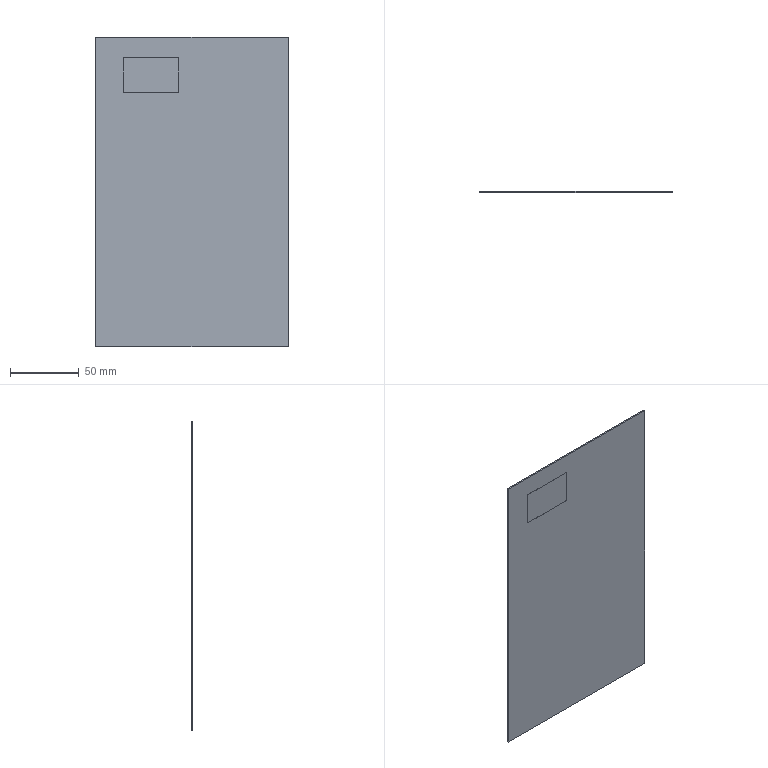Part | STEP file | Computer chassis front-side small door RR | 1 solid | 11 faces | box 140 x 1 x 225 mm | volume 31400 mm3 | plane 11
STEP:
#1=CARTESIAN_POINT('',(0.,0.,0.));
#2=DIRECTION('',(0.,0.,1.));
#3=DIRECTION('',(1.,0.,0.));
#4=AXIS2_PLACEMENT_3D('',#1,#2,#3);
#5=CARTESIAN_POINT('',(70.,1.,-112.5));
#6=VERTEX_POINT('',#5);
#7=CARTESIAN_POINT('',(-70.,1.,-112.5));
#8=VERTEX_POINT('',#7);
#9=CARTESIAN_POINT('',(0.,1.,-112.5));
#10=DIRECTION('',(-1.,0.,0.));
#11=VECTOR('',#10,1.);
#12=LINE('',#9,#11);
#13=CARTESIAN_POINT('',(0.,1.,0.));
#14=DIRECTION('',(0.,1.,0.));
#15=DIRECTION('',(0.,0.,1.));
#16=AXIS2_PLACEMENT_3D('',#13,#14,#15);
#17=PLANE('',#16);
#18=CARTESIAN_POINT('',(-112.5,0.));
#19=DIRECTION('',(0.,-1.));
#20=VECTOR('',#19,1.);
#21=LINE('',#18,#20);
#22=(GEOMETRIC_REPRESENTATION_CONTEXT(2)PARAMETRIC_REPRESENTATION_CONTEXT()REPRESENTATION_CONTEXT('',''));
#23=DEFINITIONAL_REPRESENTATION('',(#21),#22);
#24=PCURVE('',#17,#23);
#25=CARTESIAN_POINT('',(70.,0.,-112.5));
#26=DIRECTION('',(0.,0.,-1.));
#27=DIRECTION('',(-1.,0.,0.));
#28=AXIS2_PLACEMENT_3D('',#25,#26,#27);
#29=PLANE('',#28);
#30=CARTESIAN_POINT('',(70.,1.));
#31=DIRECTION('',(1.,0.));
#32=VECTOR('',#31,1.);
#33=LINE('',#30,#32);
#34=(GEOMETRIC_REPRESENTATION_CONTEXT(2)PARAMETRIC_REPRESENTATION_CONTEXT()REPRESENTATION_CONTEXT('',''));
#35=DEFINITIONAL_REPRESENTATION('',(#33),#34);
#36=PCURVE('',#29,#35);
#37=SURFACE_CURVE('',#12,(#24,#36),.PCURVE_S1.);
#38=EDGE_CURVE('',#6,#8,#37,.T.);
#39=ORIENTED_EDGE('',*,*,#38,.T.);
#40=CARTESIAN_POINT('',(-70.,1.,112.5));
#41=VERTEX_POINT('',#40);
#42=CARTESIAN_POINT('',(-70.,1.,0.));
#43=DIRECTION('',(0.,0.,1.));
#44=VECTOR('',#43,1.);
#45=LINE('',#42,#44);
#46=CARTESIAN_POINT('',(0.,-70.));
#47=DIRECTION('',(1.,0.));
#48=VECTOR('',#47,1.);
#49=LINE('',#46,#48);
#50=(GEOMETRIC_REPRESENTATION_CONTEXT(2)PARAMETRIC_REPRESENTATION_CONTEXT()REPRESENTATION_CONTEXT('',''));
#51=DEFINITIONAL_REPRESENTATION('',(#49),#50);
#52=PCURVE('',#17,#51);
#53=CARTESIAN_POINT('',(-70.,0.,-112.5));
#54=DIRECTION('',(-1.,0.,0.));
#55=DIRECTION('',(0.,0.,1.));
#56=AXIS2_PLACEMENT_3D('',#53,#54,#55);
#57=PLANE('',#56);
#58=CARTESIAN_POINT('',(112.5,1.));
#59=DIRECTION('',(1.,0.));
#60=VECTOR('',#59,1.);
#61=LINE('',#58,#60);
#62=(GEOMETRIC_REPRESENTATION_CONTEXT(2)PARAMETRIC_REPRESENTATION_CONTEXT()REPRESENTATION_CONTEXT('',''));
#63=DEFINITIONAL_REPRESENTATION('',(#61),#62);
#64=PCURVE('',#57,#63);
#65=SURFACE_CURVE('',#45,(#52,#64),.PCURVE_S1.);
#66=EDGE_CURVE('',#8,#41,#65,.T.);
#67=ORIENTED_EDGE('',*,*,#66,.T.);
#68=CARTESIAN_POINT('',(70.,1.,112.5));
#69=VERTEX_POINT('',#68);
#70=CARTESIAN_POINT('',(0.,1.,112.5));
#71=DIRECTION('',(1.,0.,0.));
#72=VECTOR('',#71,1.);
#73=LINE('',#70,#72);
#74=CARTESIAN_POINT('',(112.5,0.));
#75=DIRECTION('',(0.,1.));
#76=VECTOR('',#75,1.);
#77=LINE('',#74,#76);
#78=(GEOMETRIC_REPRESENTATION_CONTEXT(2)PARAMETRIC_REPRESENTATION_CONTEXT()REPRESENTATION_CONTEXT('',''));
#79=DEFINITIONAL_REPRESENTATION('',(#77),#78);
#80=PCURVE('',#17,#79);
#81=CARTESIAN_POINT('',(-70.,0.,112.5));
#82=DIRECTION('',(0.,0.,1.));
#83=DIRECTION('',(1.,0.,0.));
#84=AXIS2_PLACEMENT_3D('',#81,#82,#83);
#85=PLANE('',#84);
#86=CARTESIAN_POINT('',(70.,1.));
#87=DIRECTION('',(1.,0.));
#88=VECTOR('',#87,1.);
#89=LINE('',#86,#88);
#90=(GEOMETRIC_REPRESENTATION_CONTEXT(2)PARAMETRIC_REPRESENTATION_CONTEXT()REPRESENTATION_CONTEXT('',''));
#91=DEFINITIONAL_REPRESENTATION('',(#89),#90);
#92=PCURVE('',#85,#91);
#93=SURFACE_CURVE('',#73,(#80,#92),.PCURVE_S1.);
#94=EDGE_CURVE('',#41,#69,#93,.T.);
#95=ORIENTED_EDGE('',*,*,#94,.T.);
#96=CARTESIAN_POINT('',(70.,1.,0.));
#97=DIRECTION('',(0.,0.,-1.));
#98=VECTOR('',#97,1.);
#99=LINE('',#96,#98);
#100=CARTESIAN_POINT('',(0.,70.));
#101=DIRECTION('',(-1.,0.));
#102=VECTOR('',#101,1.);
#103=LINE('',#100,#102);
#104=(GEOMETRIC_REPRESENTATION_CONTEXT(2)PARAMETRIC_REPRESENTATION_CONTEXT()REPRESENTATION_CONTEXT('',''));
#105=DEFINITIONAL_REPRESENTATION('',(#103),#104);
#106=PCURVE('',#17,#105);
#107=CARTESIAN_POINT('',(70.,0.,112.5));
#108=DIRECTION('',(1.,0.,0.));
#109=DIRECTION('',(0.,0.,-1.));
#110=AXIS2_PLACEMENT_3D('',#107,#108,#109);
#111=PLANE('',#110);
#112=CARTESIAN_POINT('',(112.5,1.));
#113=DIRECTION('',(1.,0.));
#114=VECTOR('',#113,1.);
#115=LINE('',#112,#114);
#116=(GEOMETRIC_REPRESENTATION_CONTEXT(2)PARAMETRIC_REPRESENTATION_CONTEXT()REPRESENTATION_CONTEXT('',''));
#117=DEFINITIONAL_REPRESENTATION('',(#115),#116);
#118=PCURVE('',#111,#117);
#119=SURFACE_CURVE('',#99,(#106,#118),.PCURVE_S1.);
#120=EDGE_CURVE('',#69,#6,#119,.T.);
#121=ORIENTED_EDGE('',*,*,#120,.T.);
#122=EDGE_LOOP('',(#39,#67,#95,#121));
#123=FACE_BOUND('',#122,.T.);
#124=ADVANCED_FACE('',(#123),#17,.T.);
#125=CARTESIAN_POINT('',(-70.,0.,-112.5));
#126=VERTEX_POINT('',#125);
#127=CARTESIAN_POINT('',(-70.,0.,-112.5));
#128=DIRECTION('',(0.,-1.,0.));
#129=VECTOR('',#128,1.);
#130=LINE('',#127,#129);
#131=CARTESIAN_POINT('',(0.,0.));
#132=DIRECTION('',(0.,-1.));
#133=VECTOR('',#132,1.);
#134=LINE('',#131,#133);
#135=(GEOMETRIC_REPRESENTATION_CONTEXT(2)PARAMETRIC_REPRESENTATION_CONTEXT()REPRESENTATION_CONTEXT('',''));
#136=DEFINITIONAL_REPRESENTATION('',(#134),#135);
#137=PCURVE('',#57,#136);
#138=CARTESIAN_POINT('',(140.,0.));
#139=DIRECTION('',(0.,-1.));
#140=VECTOR('',#139,1.);
#141=LINE('',#138,#140);
#142=(GEOMETRIC_REPRESENTATION_CONTEXT(2)PARAMETRIC_REPRESENTATION_CONTEXT()REPRESENTATION_CONTEXT('',''));
#143=DEFINITIONAL_REPRESENTATION('',(#141),#142);
#144=PCURVE('',#29,#143);
#145=SURFACE_CURVE('',#130,(#137,#144),.PCURVE_S1.);
#146=EDGE_CURVE('',#8,#126,#145,.T.);
#147=ORIENTED_EDGE('',*,*,#146,.T.);
#148=CARTESIAN_POINT('',(-70.,0.,112.5));
#149=VERTEX_POINT('',#148);
#150=CARTESIAN_POINT('',(-70.,0.,-112.5));
#151=DIRECTION('',(0.,0.,1.));
#152=VECTOR('',#151,1.);
#153=LINE('',#150,#152);
#154=CARTESIAN_POINT('',(0.,0.));
#155=DIRECTION('',(1.,0.));
#156=VECTOR('',#155,1.);
#157=LINE('',#154,#156);
#158=(GEOMETRIC_REPRESENTATION_CONTEXT(2)PARAMETRIC_REPRESENTATION_CONTEXT()REPRESENTATION_CONTEXT('',''));
#159=DEFINITIONAL_REPRESENTATION('',(#157),#158);
#160=PCURVE('',#57,#159);
#161=CARTESIAN_POINT('',(0.,0.,0.));
#162=DIRECTION('',(0.,1.,0.));
#163=DIRECTION('',(0.,0.,1.));
#164=AXIS2_PLACEMENT_3D('',#161,#162,#163);
#165=PLANE('',#164);
#166=CARTESIAN_POINT('',(-112.5,-70.));
#167=DIRECTION('',(1.,0.));
#168=VECTOR('',#167,1.);
#169=LINE('',#166,#168);
#170=(GEOMETRIC_REPRESENTATION_CONTEXT(2)PARAMETRIC_REPRESENTATION_CONTEXT()REPRESENTATION_CONTEXT('',''));
#171=DEFINITIONAL_REPRESENTATION('',(#169),#170);
#172=PCURVE('',#165,#171);
#173=SURFACE_CURVE('',#153,(#160,#172),.PCURVE_S1.);
#174=EDGE_CURVE('',#126,#149,#173,.T.);
#175=ORIENTED_EDGE('',*,*,#174,.T.);
#176=CARTESIAN_POINT('',(-70.,0.,112.5));
#177=DIRECTION('',(0.,1.,0.));
#178=VECTOR('',#177,1.);
#179=LINE('',#176,#178);
#180=CARTESIAN_POINT('',(225.,0.));
#181=DIRECTION('',(0.,1.));
#182=VECTOR('',#181,1.);
#183=LINE('',#180,#182);
#184=(GEOMETRIC_REPRESENTATION_CONTEXT(2)PARAMETRIC_REPRESENTATION_CONTEXT()REPRESENTATION_CONTEXT('',''));
#185=DEFINITIONAL_REPRESENTATION('',(#183),#184);
#186=PCURVE('',#57,#185);
#187=CARTESIAN_POINT('',(0.,0.));
#188=DIRECTION('',(0.,1.));
#189=VECTOR('',#188,1.);
#190=LINE('',#187,#189);
#191=(GEOMETRIC_REPRESENTATION_CONTEXT(2)PARAMETRIC_REPRESENTATION_CONTEXT()REPRESENTATION_CONTEXT('',''));
#192=DEFINITIONAL_REPRESENTATION('',(#190),#191);
#193=PCURVE('',#85,#192);
#194=SURFACE_CURVE('',#179,(#186,#193),.PCURVE_S1.);
#195=EDGE_CURVE('',#149,#41,#194,.T.);
#196=ORIENTED_EDGE('',*,*,#195,.T.);
#197=ORIENTED_EDGE('',*,*,#66,.F.);
#198=EDGE_LOOP('',(#147,#175,#196,#197));
#199=FACE_BOUND('',#198,.T.);
#200=ADVANCED_FACE('',(#199),#57,.T.);
#201=CARTESIAN_POINT('',(70.,0.,-112.5));
#202=VERTEX_POINT('',#201);
#203=CARTESIAN_POINT('',(70.,0.,-112.5));
#204=DIRECTION('',(0.,-1.,0.));
#205=VECTOR('',#204,1.);
#206=LINE('',#203,#205);
#207=CARTESIAN_POINT('',(0.,0.));
#208=DIRECTION('',(0.,-1.));
#209=VECTOR('',#208,1.);
#210=LINE('',#207,#209);
#211=(GEOMETRIC_REPRESENTATION_CONTEXT(2)PARAMETRIC_REPRESENTATION_CONTEXT()REPRESENTATION_CONTEXT('',''));
#212=DEFINITIONAL_REPRESENTATION('',(#210),#211);
#213=PCURVE('',#29,#212);
#214=CARTESIAN_POINT('',(225.,0.));
#215=DIRECTION('',(0.,-1.));
#216=VECTOR('',#215,1.);
#217=LINE('',#214,#216);
#218=(GEOMETRIC_REPRESENTATION_CONTEXT(2)PARAMETRIC_REPRESENTATION_CONTEXT()REPRESENTATION_CONTEXT('',''));
#219=DEFINITIONAL_REPRESENTATION('',(#217),#218);
#220=PCURVE('',#111,#219);
#221=SURFACE_CURVE('',#206,(#213,#220),.PCURVE_S1.);
#222=EDGE_CURVE('',#6,#202,#221,.T.);
#223=ORIENTED_EDGE('',*,*,#222,.T.);
#224=CARTESIAN_POINT('',(70.,0.,-112.5));
#225=DIRECTION('',(-1.,0.,0.));
#226=VECTOR('',#225,1.);
#227=LINE('',#224,#226);
#228=CARTESIAN_POINT('',(0.,0.));
#229=DIRECTION('',(1.,0.));
#230=VECTOR('',#229,1.);
#231=LINE('',#228,#230);
#232=(GEOMETRIC_REPRESENTATION_CONTEXT(2)PARAMETRIC_REPRESENTATION_CONTEXT()REPRESENTATION_CONTEXT('',''));
#233=DEFINITIONAL_REPRESENTATION('',(#231),#232);
#234=PCURVE('',#29,#233);
#235=CARTESIAN_POINT('',(-112.5,70.));
#236=DIRECTION('',(0.,-1.));
#237=VECTOR('',#236,1.);
#238=LINE('',#235,#237);
#239=(GEOMETRIC_REPRESENTATION_CONTEXT(2)PARAMETRIC_REPRESENTATION_CONTEXT()REPRESENTATION_CONTEXT('',''));
#240=DEFINITIONAL_REPRESENTATION('',(#238),#239);
#241=PCURVE('',#165,#240);
#242=SURFACE_CURVE('',#227,(#234,#241),.PCURVE_S1.);
#243=EDGE_CURVE('',#202,#126,#242,.T.);
#244=ORIENTED_EDGE('',*,*,#243,.T.);
#245=ORIENTED_EDGE('',*,*,#146,.F.);
#246=ORIENTED_EDGE('',*,*,#38,.F.);
#247=EDGE_LOOP('',(#223,#244,#245,#246));
#248=FACE_BOUND('',#247,.T.);
#249=ADVANCED_FACE('',(#248),#29,.T.);
#250=CARTESIAN_POINT('',(70.,0.,112.5));
#251=VERTEX_POINT('',#250);
#252=CARTESIAN_POINT('',(70.,0.,112.5));
#253=DIRECTION('',(0.,-1.,0.));
#254=VECTOR('',#253,1.);
#255=LINE('',#252,#254);
#256=CARTESIAN_POINT('',(0.,0.));
#257=DIRECTION('',(0.,-1.));
#258=VECTOR('',#257,1.);
#259=LINE('',#256,#258);
#260=(GEOMETRIC_REPRESENTATION_CONTEXT(2)PARAMETRIC_REPRESENTATION_CONTEXT()REPRESENTATION_CONTEXT('',''));
#261=DEFINITIONAL_REPRESENTATION('',(#259),#260);
#262=PCURVE('',#111,#261);
#263=CARTESIAN_POINT('',(140.,0.));
#264=DIRECTION('',(0.,-1.));
#265=VECTOR('',#264,1.);
#266=LINE('',#263,#265);
#267=(GEOMETRIC_REPRESENTATION_CONTEXT(2)PARAMETRIC_REPRESENTATION_CONTEXT()REPRESENTATION_CONTEXT('',''));
#268=DEFINITIONAL_REPRESENTATION('',(#266),#267);
#269=PCURVE('',#85,#268);
#270=SURFACE_CURVE('',#255,(#262,#269),.PCURVE_S1.);
#271=EDGE_CURVE('',#69,#251,#270,.T.);
#272=ORIENTED_EDGE('',*,*,#271,.T.);
#273=CARTESIAN_POINT('',(70.,0.,112.5));
#274=DIRECTION('',(0.,0.,-1.));
#275=VECTOR('',#274,1.);
#276=LINE('',#273,#275);
#277=CARTESIAN_POINT('',(0.,0.));
#278=DIRECTION('',(1.,0.));
#279=VECTOR('',#278,1.);
#280=LINE('',#277,#279);
#281=(GEOMETRIC_REPRESENTATION_CONTEXT(2)PARAMETRIC_REPRESENTATION_CONTEXT()REPRESENTATION_CONTEXT('',''));
#282=DEFINITIONAL_REPRESENTATION('',(#280),#281);
#283=PCURVE('',#111,#282);
#284=CARTESIAN_POINT('',(112.5,70.));
#285=DIRECTION('',(-1.,0.));
#286=VECTOR('',#285,1.);
#287=LINE('',#284,#286);
#288=(GEOMETRIC_REPRESENTATION_CONTEXT(2)PARAMETRIC_REPRESENTATION_CONTEXT()REPRESENTATION_CONTEXT('',''));
#289=DEFINITIONAL_REPRESENTATION('',(#287),#288);
#290=PCURVE('',#165,#289);
#291=SURFACE_CURVE('',#276,(#283,#290),.PCURVE_S1.);
#292=EDGE_CURVE('',#251,#202,#291,.T.);
#293=ORIENTED_EDGE('',*,*,#292,.T.);
#294=ORIENTED_EDGE('',*,*,#222,.F.);
#295=ORIENTED_EDGE('',*,*,#120,.F.);
#296=EDGE_LOOP('',(#272,#293,#294,#295));
#297=FACE_BOUND('',#296,.T.);
#298=ADVANCED_FACE('',(#297),#111,.T.);
#299=ORIENTED_EDGE('',*,*,#195,.F.);
#300=CARTESIAN_POINT('',(-70.,0.,112.5));
#301=DIRECTION('',(1.,0.,0.));
#302=VECTOR('',#301,1.);
#303=LINE('',#300,#302);
#304=CARTESIAN_POINT('',(0.,0.));
#305=DIRECTION('',(1.,0.));
#306=VECTOR('',#305,1.);
#307=LINE('',#304,#306);
#308=(GEOMETRIC_REPRESENTATION_CONTEXT(2)PARAMETRIC_REPRESENTATION_CONTEXT()REPRESENTATION_CONTEXT('',''));
#309=DEFINITIONAL_REPRESENTATION('',(#307),#308);
#310=PCURVE('',#85,#309);
#311=CARTESIAN_POINT('',(112.5,-70.));
#312=DIRECTION('',(0.,1.));
#313=VECTOR('',#312,1.);
#314=LINE('',#311,#313);
#315=(GEOMETRIC_REPRESENTATION_CONTEXT(2)PARAMETRIC_REPRESENTATION_CONTEXT()REPRESENTATION_CONTEXT('',''));
#316=DEFINITIONAL_REPRESENTATION('',(#314),#315);
#317=PCURVE('',#165,#316);
#318=SURFACE_CURVE('',#303,(#310,#317),.PCURVE_S1.);
#319=EDGE_CURVE('',#149,#251,#318,.T.);
#320=ORIENTED_EDGE('',*,*,#319,.T.);
#321=ORIENTED_EDGE('',*,*,#271,.F.);
#322=ORIENTED_EDGE('',*,*,#94,.F.);
#323=EDGE_LOOP('',(#299,#320,#321,#322));
#324=FACE_BOUND('',#323,.T.);
#325=ADVANCED_FACE('',(#324),#85,.T.);
#326=CARTESIAN_POINT('',(-50.,0.,97.5));
#327=VERTEX_POINT('',#326);
#328=CARTESIAN_POINT('',(-50.,0.,72.5));
#329=VERTEX_POINT('',#328);
#330=CARTESIAN_POINT('',(-50.,0.,0.));
#331=DIRECTION('',(0.,0.,-1.));
#332=VECTOR('',#331,1.);
#333=LINE('',#330,#332);
#334=CARTESIAN_POINT('',(0.,-50.));
#335=DIRECTION('',(-1.,0.));
#336=VECTOR('',#335,1.);
#337=LINE('',#334,#336);
#338=(GEOMETRIC_REPRESENTATION_CONTEXT(2)PARAMETRIC_REPRESENTATION_CONTEXT()REPRESENTATION_CONTEXT('',''));
#339=DEFINITIONAL_REPRESENTATION('',(#337),#338);
#340=PCURVE('',#165,#339);
#341=CARTESIAN_POINT('',(-50.,0.,97.5));
#342=DIRECTION('',(-1.,0.,0.));
#343=DIRECTION('',(0.,0.,1.));
#344=AXIS2_PLACEMENT_3D('',#341,#342,#343);
#345=PLANE('',#344);
#346=CARTESIAN_POINT('',(-97.5,0.));
#347=DIRECTION('',(-1.,0.));
#348=VECTOR('',#347,1.);
#349=LINE('',#346,#348);
#350=(GEOMETRIC_REPRESENTATION_CONTEXT(2)PARAMETRIC_REPRESENTATION_CONTEXT()REPRESENTATION_CONTEXT('',''));
#351=DEFINITIONAL_REPRESENTATION('',(#349),#350);
#352=PCURVE('',#345,#351);
#353=SURFACE_CURVE('',#333,(#340,#352),.PCURVE_S1.);
#354=EDGE_CURVE('',#327,#329,#353,.T.);
#355=ORIENTED_EDGE('',*,*,#354,.F.);
#356=CARTESIAN_POINT('',(-10.,0.,97.5));
#357=VERTEX_POINT('',#356);
#358=CARTESIAN_POINT('',(0.,0.,97.5));
#359=DIRECTION('',(-1.,0.,0.));
#360=VECTOR('',#359,1.);
#361=LINE('',#358,#360);
#362=CARTESIAN_POINT('',(97.5,0.));
#363=DIRECTION('',(0.,-1.));
#364=VECTOR('',#363,1.);
#365=LINE('',#362,#364);
#366=(GEOMETRIC_REPRESENTATION_CONTEXT(2)PARAMETRIC_REPRESENTATION_CONTEXT()REPRESENTATION_CONTEXT('',''));
#367=DEFINITIONAL_REPRESENTATION('',(#365),#366);
#368=PCURVE('',#165,#367);
#369=CARTESIAN_POINT('',(-10.,0.,97.5));
#370=DIRECTION('',(0.,0.,1.));
#371=DIRECTION('',(1.,0.,0.));
#372=AXIS2_PLACEMENT_3D('',#369,#370,#371);
#373=PLANE('',#372);
#374=CARTESIAN_POINT('',(10.,0.));
#375=DIRECTION('',(-1.,0.));
#376=VECTOR('',#375,1.);
#377=LINE('',#374,#376);
#378=(GEOMETRIC_REPRESENTATION_CONTEXT(2)PARAMETRIC_REPRESENTATION_CONTEXT()REPRESENTATION_CONTEXT('',''));
#379=DEFINITIONAL_REPRESENTATION('',(#377),#378);
#380=PCURVE('',#373,#379);
#381=SURFACE_CURVE('',#361,(#368,#380),.PCURVE_S1.);
#382=EDGE_CURVE('',#357,#327,#381,.T.);
#383=ORIENTED_EDGE('',*,*,#382,.F.);
#384=CARTESIAN_POINT('',(-10.,0.,72.5));
#385=VERTEX_POINT('',#384);
#386=CARTESIAN_POINT('',(-10.,0.,0.));
#387=DIRECTION('',(0.,0.,1.));
#388=VECTOR('',#387,1.);
#389=LINE('',#386,#388);
#390=CARTESIAN_POINT('',(0.,-10.));
#391=DIRECTION('',(1.,0.));
#392=VECTOR('',#391,1.);
#393=LINE('',#390,#392);
#394=(GEOMETRIC_REPRESENTATION_CONTEXT(2)PARAMETRIC_REPRESENTATION_CONTEXT()REPRESENTATION_CONTEXT('',''));
#395=DEFINITIONAL_REPRESENTATION('',(#393),#394);
#396=PCURVE('',#165,#395);
#397=CARTESIAN_POINT('',(-10.,0.,72.5));
#398=DIRECTION('',(1.,0.,0.));
#399=DIRECTION('',(0.,0.,-1.));
#400=AXIS2_PLACEMENT_3D('',#397,#398,#399);
#401=PLANE('',#400);
#402=CARTESIAN_POINT('',(72.5,0.));
#403=DIRECTION('',(-1.,0.));
#404=VECTOR('',#403,1.);
#405=LINE('',#402,#404);
#406=(GEOMETRIC_REPRESENTATION_CONTEXT(2)PARAMETRIC_REPRESENTATION_CONTEXT()REPRESENTATION_CONTEXT('',''));
#407=DEFINITIONAL_REPRESENTATION('',(#405),#406);
#408=PCURVE('',#401,#407);
#409=SURFACE_CURVE('',#389,(#396,#408),.PCURVE_S1.);
#410=EDGE_CURVE('',#385,#357,#409,.T.);
#411=ORIENTED_EDGE('',*,*,#410,.F.);
#412=CARTESIAN_POINT('',(0.,0.,72.5));
#413=DIRECTION('',(1.,0.,0.));
#414=VECTOR('',#413,1.);
#415=LINE('',#412,#414);
#416=CARTESIAN_POINT('',(72.5,0.));
#417=DIRECTION('',(0.,1.));
#418=VECTOR('',#417,1.);
#419=LINE('',#416,#418);
#420=(GEOMETRIC_REPRESENTATION_CONTEXT(2)PARAMETRIC_REPRESENTATION_CONTEXT()REPRESENTATION_CONTEXT('',''));
#421=DEFINITIONAL_REPRESENTATION('',(#419),#420);
#422=PCURVE('',#165,#421);
#423=CARTESIAN_POINT('',(-50.,0.,72.5));
#424=DIRECTION('',(0.,0.,-1.));
#425=DIRECTION('',(-1.,0.,0.));
#426=AXIS2_PLACEMENT_3D('',#423,#424,#425);
#427=PLANE('',#426);
#428=CARTESIAN_POINT('',(-50.,0.));
#429=DIRECTION('',(-1.,0.));
#430=VECTOR('',#429,1.);
#431=LINE('',#428,#430);
#432=(GEOMETRIC_REPRESENTATION_CONTEXT(2)PARAMETRIC_REPRESENTATION_CONTEXT()REPRESENTATION_CONTEXT('',''));
#433=DEFINITIONAL_REPRESENTATION('',(#431),#432);
#434=PCURVE('',#427,#433);
#435=SURFACE_CURVE('',#415,(#422,#434),.PCURVE_S1.);
#436=EDGE_CURVE('',#329,#385,#435,.T.);
#437=ORIENTED_EDGE('',*,*,#436,.F.);
#438=EDGE_LOOP('',(#355,#383,#411,#437));
#439=FACE_BOUND('',#438,.T.);
#440=ORIENTED_EDGE('',*,*,#292,.F.);
#441=ORIENTED_EDGE('',*,*,#319,.F.);
#442=ORIENTED_EDGE('',*,*,#174,.F.);
#443=ORIENTED_EDGE('',*,*,#243,.F.);
#444=EDGE_LOOP('',(#440,#441,#442,#443));
#445=FACE_BOUND('',#444,.T.);
#446=ADVANCED_FACE('',(#439,#445),#165,.F.);
#447=CARTESIAN_POINT('',(-50.,0.1,72.5));
#448=VERTEX_POINT('',#447);
#449=CARTESIAN_POINT('',(-10.,0.1,72.5));
#450=VERTEX_POINT('',#449);
#451=CARTESIAN_POINT('',(-50.,0.1,72.5));
#452=DIRECTION('',(1.,0.,0.));
#453=VECTOR('',#452,1.);
#454=LINE('',#451,#453);
#455=CARTESIAN_POINT('',(0.,0.1));
#456=DIRECTION('',(-1.,0.));
#457=VECTOR('',#456,1.);
#458=LINE('',#455,#457);
#459=(GEOMETRIC_REPRESENTATION_CONTEXT(2)PARAMETRIC_REPRESENTATION_CONTEXT()REPRESENTATION_CONTEXT('',''));
#460=DEFINITIONAL_REPRESENTATION('',(#458),#459);
#461=PCURVE('',#427,#460);
#462=CARTESIAN_POINT('',(0.,0.1,0.));
#463=DIRECTION('',(0.,-1.,0.));
#464=DIRECTION('',(0.,0.,-1.));
#465=AXIS2_PLACEMENT_3D('',#462,#463,#464);
#466=PLANE('',#465);
#467=CARTESIAN_POINT('',(-72.5,-50.));
#468=DIRECTION('',(0.,1.));
#469=VECTOR('',#468,1.);
#470=LINE('',#467,#469);
#471=(GEOMETRIC_REPRESENTATION_CONTEXT(2)PARAMETRIC_REPRESENTATION_CONTEXT()REPRESENTATION_CONTEXT('',''));
#472=DEFINITIONAL_REPRESENTATION('',(#470),#471);
#473=PCURVE('',#466,#472);
#474=SURFACE_CURVE('',#454,(#461,#473),.PCURVE_S1.);
#475=EDGE_CURVE('',#448,#450,#474,.T.);
#476=ORIENTED_EDGE('',*,*,#475,.F.);
#477=CARTESIAN_POINT('',(-50.,0.,72.5));
#478=DIRECTION('',(0.,1.,0.));
#479=VECTOR('',#478,1.);
#480=LINE('',#477,#479);
#481=CARTESIAN_POINT('',(0.,0.));
#482=DIRECTION('',(0.,1.));
#483=VECTOR('',#482,1.);
#484=LINE('',#481,#483);
#485=(GEOMETRIC_REPRESENTATION_CONTEXT(2)PARAMETRIC_REPRESENTATION_CONTEXT()REPRESENTATION_CONTEXT('',''));
#486=DEFINITIONAL_REPRESENTATION('',(#484),#485);
#487=PCURVE('',#427,#486);
#488=CARTESIAN_POINT('',(-25.,0.));
#489=DIRECTION('',(0.,1.));
#490=VECTOR('',#489,1.);
#491=LINE('',#488,#490);
#492=(GEOMETRIC_REPRESENTATION_CONTEXT(2)PARAMETRIC_REPRESENTATION_CONTEXT()REPRESENTATION_CONTEXT('',''));
#493=DEFINITIONAL_REPRESENTATION('',(#491),#492);
#494=PCURVE('',#345,#493);
#495=SURFACE_CURVE('',#480,(#487,#494),.PCURVE_S1.);
#496=EDGE_CURVE('',#329,#448,#495,.T.);
#497=ORIENTED_EDGE('',*,*,#496,.F.);
#498=ORIENTED_EDGE('',*,*,#436,.T.);
#499=CARTESIAN_POINT('',(-10.,0.,72.5));
#500=DIRECTION('',(0.,-1.,0.));
#501=VECTOR('',#500,1.);
#502=LINE('',#499,#501);
#503=CARTESIAN_POINT('',(-40.,0.));
#504=DIRECTION('',(0.,-1.));
#505=VECTOR('',#504,1.);
#506=LINE('',#503,#505);
#507=(GEOMETRIC_REPRESENTATION_CONTEXT(2)PARAMETRIC_REPRESENTATION_CONTEXT()REPRESENTATION_CONTEXT('',''));
#508=DEFINITIONAL_REPRESENTATION('',(#506),#507);
#509=PCURVE('',#427,#508);
#510=CARTESIAN_POINT('',(0.,0.));
#511=DIRECTION('',(0.,-1.));
#512=VECTOR('',#511,1.);
#513=LINE('',#510,#512);
#514=(GEOMETRIC_REPRESENTATION_CONTEXT(2)PARAMETRIC_REPRESENTATION_CONTEXT()REPRESENTATION_CONTEXT('',''));
#515=DEFINITIONAL_REPRESENTATION('',(#513),#514);
#516=PCURVE('',#401,#515);
#517=SURFACE_CURVE('',#502,(#509,#516),.PCURVE_S1.);
#518=EDGE_CURVE('',#450,#385,#517,.T.);
#519=ORIENTED_EDGE('',*,*,#518,.F.);
#520=EDGE_LOOP('',(#476,#497,#498,#519));
#521=FACE_BOUND('',#520,.T.);
#522=ADVANCED_FACE('',(#521),#427,.F.);
#523=CARTESIAN_POINT('',(-50.,0.1,97.5));
#524=VERTEX_POINT('',#523);
#525=CARTESIAN_POINT('',(-50.,0.1,97.5));
#526=DIRECTION('',(0.,0.,-1.));
#527=VECTOR('',#526,1.);
#528=LINE('',#525,#527);
#529=CARTESIAN_POINT('',(0.,0.1));
#530=DIRECTION('',(-1.,0.));
#531=VECTOR('',#530,1.);
#532=LINE('',#529,#531);
#533=(GEOMETRIC_REPRESENTATION_CONTEXT(2)PARAMETRIC_REPRESENTATION_CONTEXT()REPRESENTATION_CONTEXT('',''));
#534=DEFINITIONAL_REPRESENTATION('',(#532),#533);
#535=PCURVE('',#345,#534);
#536=CARTESIAN_POINT('',(-97.5,-50.));
#537=DIRECTION('',(1.,0.));
#538=VECTOR('',#537,1.);
#539=LINE('',#536,#538);
#540=(GEOMETRIC_REPRESENTATION_CONTEXT(2)PARAMETRIC_REPRESENTATION_CONTEXT()REPRESENTATION_CONTEXT('',''));
#541=DEFINITIONAL_REPRESENTATION('',(#539),#540);
#542=PCURVE('',#466,#541);
#543=SURFACE_CURVE('',#528,(#535,#542),.PCURVE_S1.);
#544=EDGE_CURVE('',#524,#448,#543,.T.);
#545=ORIENTED_EDGE('',*,*,#544,.F.);
#546=CARTESIAN_POINT('',(-50.,0.,97.5));
#547=DIRECTION('',(0.,1.,0.));
#548=VECTOR('',#547,1.);
#549=LINE('',#546,#548);
#550=CARTESIAN_POINT('',(0.,0.));
#551=DIRECTION('',(0.,1.));
#552=VECTOR('',#551,1.);
#553=LINE('',#550,#552);
#554=(GEOMETRIC_REPRESENTATION_CONTEXT(2)PARAMETRIC_REPRESENTATION_CONTEXT()REPRESENTATION_CONTEXT('',''));
#555=DEFINITIONAL_REPRESENTATION('',(#553),#554);
#556=PCURVE('',#345,#555);
#557=CARTESIAN_POINT('',(-40.,0.));
#558=DIRECTION('',(0.,1.));
#559=VECTOR('',#558,1.);
#560=LINE('',#557,#559);
#561=(GEOMETRIC_REPRESENTATION_CONTEXT(2)PARAMETRIC_REPRESENTATION_CONTEXT()REPRESENTATION_CONTEXT('',''));
#562=DEFINITIONAL_REPRESENTATION('',(#560),#561);
#563=PCURVE('',#373,#562);
#564=SURFACE_CURVE('',#549,(#556,#563),.PCURVE_S1.);
#565=EDGE_CURVE('',#327,#524,#564,.T.);
#566=ORIENTED_EDGE('',*,*,#565,.F.);
#567=ORIENTED_EDGE('',*,*,#354,.T.);
#568=ORIENTED_EDGE('',*,*,#496,.T.);
#569=EDGE_LOOP('',(#545,#566,#567,#568));
#570=FACE_BOUND('',#569,.T.);
#571=ADVANCED_FACE('',(#570),#345,.F.);
#572=CARTESIAN_POINT('',(-10.,0.1,97.5));
#573=VERTEX_POINT('',#572);
#574=CARTESIAN_POINT('',(-10.,0.1,97.5));
#575=DIRECTION('',(-1.,0.,0.));
#576=VECTOR('',#575,1.);
#577=LINE('',#574,#576);
#578=CARTESIAN_POINT('',(0.,0.1));
#579=DIRECTION('',(-1.,0.));
#580=VECTOR('',#579,1.);
#581=LINE('',#578,#580);
#582=(GEOMETRIC_REPRESENTATION_CONTEXT(2)PARAMETRIC_REPRESENTATION_CONTEXT()REPRESENTATION_CONTEXT('',''));
#583=DEFINITIONAL_REPRESENTATION('',(#581),#582);
#584=PCURVE('',#373,#583);
#585=CARTESIAN_POINT('',(-97.5,-10.));
#586=DIRECTION('',(0.,-1.));
#587=VECTOR('',#586,1.);
#588=LINE('',#585,#587);
#589=(GEOMETRIC_REPRESENTATION_CONTEXT(2)PARAMETRIC_REPRESENTATION_CONTEXT()REPRESENTATION_CONTEXT('',''));
#590=DEFINITIONAL_REPRESENTATION('',(#588),#589);
#591=PCURVE('',#466,#590);
#592=SURFACE_CURVE('',#577,(#584,#591),.PCURVE_S1.);
#593=EDGE_CURVE('',#573,#524,#592,.T.);
#594=ORIENTED_EDGE('',*,*,#593,.F.);
#595=CARTESIAN_POINT('',(-10.,0.,97.5));
#596=DIRECTION('',(0.,1.,0.));
#597=VECTOR('',#596,1.);
#598=LINE('',#595,#597);
#599=CARTESIAN_POINT('',(0.,0.));
#600=DIRECTION('',(0.,1.));
#601=VECTOR('',#600,1.);
#602=LINE('',#599,#601);
#603=(GEOMETRIC_REPRESENTATION_CONTEXT(2)PARAMETRIC_REPRESENTATION_CONTEXT()REPRESENTATION_CONTEXT('',''));
#604=DEFINITIONAL_REPRESENTATION('',(#602),#603);
#605=PCURVE('',#373,#604);
#606=CARTESIAN_POINT('',(-25.,0.));
#607=DIRECTION('',(0.,1.));
#608=VECTOR('',#607,1.);
#609=LINE('',#606,#608);
#610=(GEOMETRIC_REPRESENTATION_CONTEXT(2)PARAMETRIC_REPRESENTATION_CONTEXT()REPRESENTATION_CONTEXT('',''));
#611=DEFINITIONAL_REPRESENTATION('',(#609),#610);
#612=PCURVE('',#401,#611);
#613=SURFACE_CURVE('',#598,(#605,#612),.PCURVE_S1.);
#614=EDGE_CURVE('',#357,#573,#613,.T.);
#615=ORIENTED_EDGE('',*,*,#614,.F.);
#616=ORIENTED_EDGE('',*,*,#382,.T.);
#617=ORIENTED_EDGE('',*,*,#565,.T.);
#618=EDGE_LOOP('',(#594,#615,#616,#617));
#619=FACE_BOUND('',#618,.T.);
#620=ADVANCED_FACE('',(#619),#373,.F.);
#621=CARTESIAN_POINT('',(-10.,0.1,72.5));
#622=DIRECTION('',(0.,0.,1.));
#623=VECTOR('',#622,1.);
#624=LINE('',#621,#623);
#625=CARTESIAN_POINT('',(0.,0.1));
#626=DIRECTION('',(-1.,0.));
#627=VECTOR('',#626,1.);
#628=LINE('',#625,#627);
#629=(GEOMETRIC_REPRESENTATION_CONTEXT(2)PARAMETRIC_REPRESENTATION_CONTEXT()REPRESENTATION_CONTEXT('',''));
#630=DEFINITIONAL_REPRESENTATION('',(#628),#629);
#631=PCURVE('',#401,#630);
#632=CARTESIAN_POINT('',(-72.5,-10.));
#633=DIRECTION('',(-1.,0.));
#634=VECTOR('',#633,1.);
#635=LINE('',#632,#634);
#636=(GEOMETRIC_REPRESENTATION_CONTEXT(2)PARAMETRIC_REPRESENTATION_CONTEXT()REPRESENTATION_CONTEXT('',''));
#637=DEFINITIONAL_REPRESENTATION('',(#635),#636);
#638=PCURVE('',#466,#637);
#639=SURFACE_CURVE('',#624,(#631,#638),.PCURVE_S1.);
#640=EDGE_CURVE('',#450,#573,#639,.T.);
#641=ORIENTED_EDGE('',*,*,#640,.F.);
#642=ORIENTED_EDGE('',*,*,#518,.T.);
#643=ORIENTED_EDGE('',*,*,#410,.T.);
#644=ORIENTED_EDGE('',*,*,#614,.T.);
#645=EDGE_LOOP('',(#641,#642,#643,#644));
#646=FACE_BOUND('',#645,.T.);
#647=ADVANCED_FACE('',(#646),#401,.F.);
#648=ORIENTED_EDGE('',*,*,#475,.T.);
#649=ORIENTED_EDGE('',*,*,#640,.T.);
#650=ORIENTED_EDGE('',*,*,#593,.T.);
#651=ORIENTED_EDGE('',*,*,#544,.T.);
#652=EDGE_LOOP('',(#648,#649,#650,#651));
#653=FACE_BOUND('',#652,.T.);
#654=ADVANCED_FACE('',(#653),#466,.T.);
#655=CLOSED_SHELL('',(#124,#200,#249,#298,#325,#446,#522,#571,#620,#647,#654));
#656=MANIFOLD_SOLID_BREP('',#655);
#657=(LENGTH_UNIT()NAMED_UNIT(*)SI_UNIT(.MILLI.,.METRE.));
#658=UNCERTAINTY_MEASURE_WITH_UNIT(LENGTH_MEASURE(0.0000001),#657,'','');
#659=(NAMED_UNIT(*)PLANE_ANGLE_UNIT()SI_UNIT($,.RADIAN.));
#660=(NAMED_UNIT(*)SI_UNIT($,.STERADIAN.)SOLID_ANGLE_UNIT());
#661=(GEOMETRIC_REPRESENTATION_CONTEXT(3)GLOBAL_UNCERTAINTY_ASSIGNED_CONTEXT((#658))GLOBAL_UNIT_ASSIGNED_CONTEXT((#657,#659,#660))REPRESENTATION_CONTEXT('',''));
#662=ADVANCED_BREP_SHAPE_REPRESENTATION('',(#4,#656),#661);